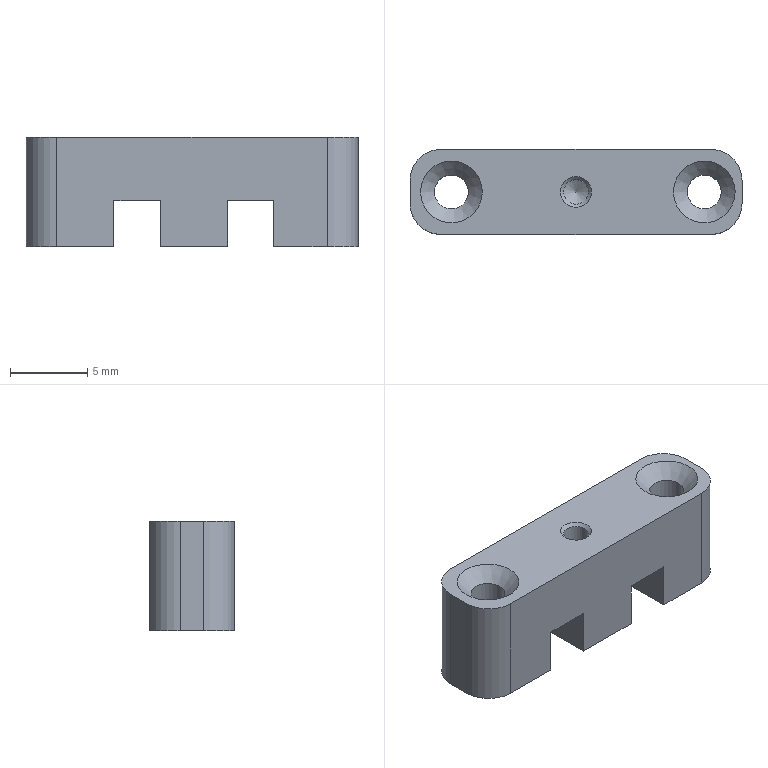Part | STEP file | Driver amplifier partition | 1 solid | 27 faces | box 21.48 x 5.5 x 7.1 mm | volume 643.148 mm3 | plane 14 | cylinder 7 | cone 6 | commonest cylinder face diameters 4 x4 2.2 x2 1.6 x1